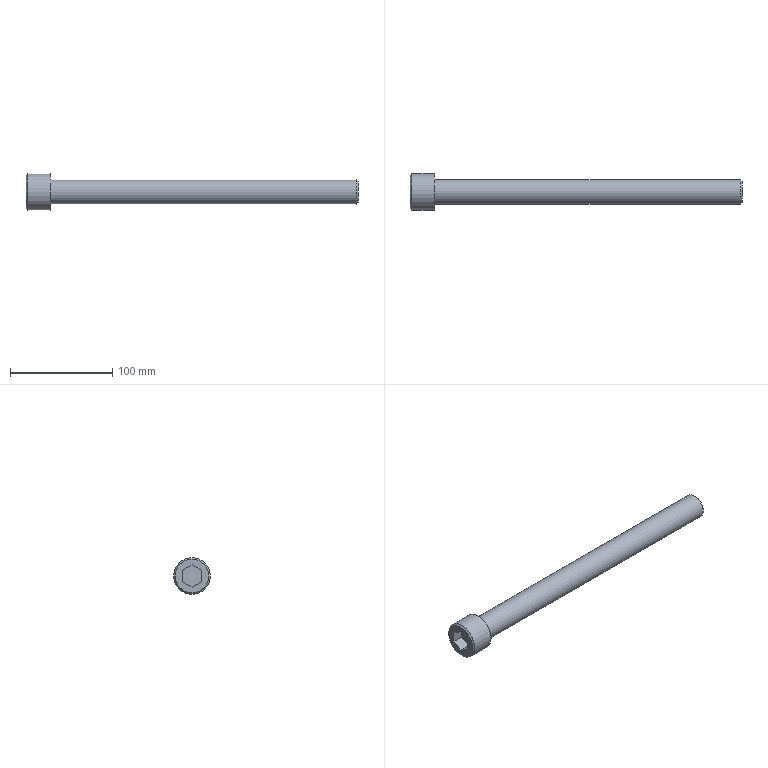Part | STEP file | solid 53 | 1 solid | 14 faces | box 325 x 36 x 36 mm | volume 156954 mm3 | plane 10 | cylinder 2 | cone 2 | commonest cylinder face diameters 24 x1 36 x1